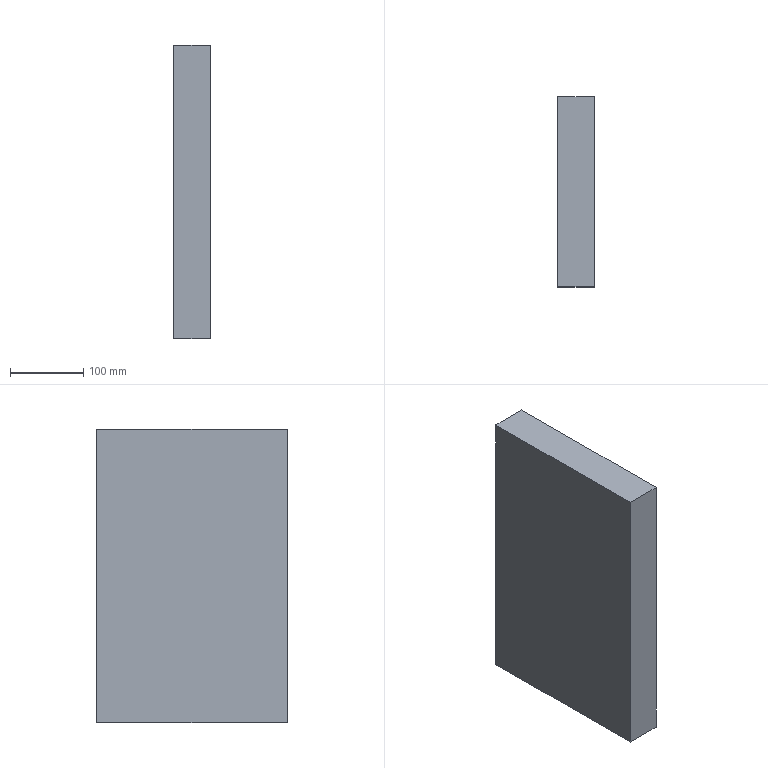Part | STEP file | 1 solid | 6 faces | box 50 x 259.164 x 400 mm | volume 5183281 mm3 | plane 6
STEP:
#1=CARTESIAN_POINT('',(0.,0.,0.));
#2=DIRECTION('',(0.,0.,1.));
#3=DIRECTION('',(1.,0.,0.));
#4=AXIS2_PLACEMENT_3D('',#1,#2,#3);
#5=CARTESIAN_POINT('',(-600.,-240.836,-56.359));
#6=VERTEX_POINT('',#5);
#7=CARTESIAN_POINT('',(-600.,-500.,-56.359));
#8=VERTEX_POINT('',#7);
#9=CARTESIAN_POINT('',(-600.,-240.836,-56.359));
#10=DIRECTION('',(0.,-1.,0.));
#11=VECTOR('',#10,1.);
#12=LINE('',#9,#11);
#13=CARTESIAN_POINT('',(-550.,-240.836,-56.359));
#14=DIRECTION('',(0.,0.,-1.));
#15=DIRECTION('',(-1.,0.,0.));
#16=AXIS2_PLACEMENT_3D('',#13,#14,#15);
#17=PLANE('',#16);
#18=CARTESIAN_POINT('',(50.,0.));
#19=DIRECTION('',(0.,-1.));
#20=VECTOR('',#19,1.);
#21=LINE('',#18,#20);
#22=(GEOMETRIC_REPRESENTATION_CONTEXT(2)PARAMETRIC_REPRESENTATION_CONTEXT()REPRESENTATION_CONTEXT('',''));
#23=DEFINITIONAL_REPRESENTATION('',(#21),#22);
#24=PCURVE('',#17,#23);
#25=CARTESIAN_POINT('',(-600.,0.,143.641));
#26=DIRECTION('',(-1.,0.,0.));
#27=DIRECTION('',(0.,0.,1.));
#28=AXIS2_PLACEMENT_3D('',#25,#26,#27);
#29=PLANE('',#28);
#30=CARTESIAN_POINT('',(-200.,-240.836));
#31=DIRECTION('',(0.,-1.));
#32=VECTOR('',#31,1.);
#33=LINE('',#30,#32);
#34=(GEOMETRIC_REPRESENTATION_CONTEXT(2)PARAMETRIC_REPRESENTATION_CONTEXT()REPRESENTATION_CONTEXT('',''));
#35=DEFINITIONAL_REPRESENTATION('',(#33),#34);
#36=PCURVE('',#29,#35);
#37=SURFACE_CURVE('',#12,(#24,#36),.PCURVE_S1.);
#38=EDGE_CURVE('',#6,#8,#37,.T.);
#39=ORIENTED_EDGE('',*,*,#38,.F.);
#40=CARTESIAN_POINT('',(-550.,-240.836,-56.359));
#41=VERTEX_POINT('',#40);
#42=CARTESIAN_POINT('',(-550.,-240.836,-56.359));
#43=DIRECTION('',(-1.,0.,0.));
#44=VECTOR('',#43,1.);
#45=LINE('',#42,#44);
#46=CARTESIAN_POINT('',(0.,0.));
#47=DIRECTION('',(1.,0.));
#48=VECTOR('',#47,1.);
#49=LINE('',#46,#48);
#50=(GEOMETRIC_REPRESENTATION_CONTEXT(2)PARAMETRIC_REPRESENTATION_CONTEXT()REPRESENTATION_CONTEXT('',''));
#51=DEFINITIONAL_REPRESENTATION('',(#49),#50);
#52=PCURVE('',#17,#51);
#53=CARTESIAN_POINT('',(-550.,-240.836,-56.359));
#54=DIRECTION('',(0.,1.,0.));
#55=DIRECTION('',(0.,0.,1.));
#56=AXIS2_PLACEMENT_3D('',#53,#54,#55);
#57=PLANE('',#56);
#58=CARTESIAN_POINT('',(0.,0.));
#59=DIRECTION('',(0.,-1.));
#60=VECTOR('',#59,1.);
#61=LINE('',#58,#60);
#62=(GEOMETRIC_REPRESENTATION_CONTEXT(2)PARAMETRIC_REPRESENTATION_CONTEXT()REPRESENTATION_CONTEXT('',''));
#63=DEFINITIONAL_REPRESENTATION('',(#61),#62);
#64=PCURVE('',#57,#63);
#65=SURFACE_CURVE('',#45,(#52,#64),.PCURVE_S1.);
#66=EDGE_CURVE('',#41,#6,#65,.T.);
#67=ORIENTED_EDGE('',*,*,#66,.F.);
#68=CARTESIAN_POINT('',(-550.,-500.,-56.359));
#69=VERTEX_POINT('',#68);
#70=CARTESIAN_POINT('',(-550.,-240.836,-56.359));
#71=DIRECTION('',(0.,-1.,0.));
#72=VECTOR('',#71,1.);
#73=LINE('',#70,#72);
#74=CARTESIAN_POINT('',(0.,0.));
#75=DIRECTION('',(0.,-1.));
#76=VECTOR('',#75,1.);
#77=LINE('',#74,#76);
#78=(GEOMETRIC_REPRESENTATION_CONTEXT(2)PARAMETRIC_REPRESENTATION_CONTEXT()REPRESENTATION_CONTEXT('',''));
#79=DEFINITIONAL_REPRESENTATION('',(#77),#78);
#80=PCURVE('',#17,#79);
#81=CARTESIAN_POINT('',(-550.,0.,143.641));
#82=DIRECTION('',(-1.,0.,0.));
#83=DIRECTION('',(0.,0.,1.));
#84=AXIS2_PLACEMENT_3D('',#81,#82,#83);
#85=PLANE('',#84);
#86=CARTESIAN_POINT('',(-200.,-240.836));
#87=DIRECTION('',(0.,-1.));
#88=VECTOR('',#87,1.);
#89=LINE('',#86,#88);
#90=(GEOMETRIC_REPRESENTATION_CONTEXT(2)PARAMETRIC_REPRESENTATION_CONTEXT()REPRESENTATION_CONTEXT('',''));
#91=DEFINITIONAL_REPRESENTATION('',(#89),#90);
#92=PCURVE('',#85,#91);
#93=SURFACE_CURVE('',#73,(#80,#92),.PCURVE_S1.);
#94=EDGE_CURVE('',#41,#69,#93,.T.);
#95=ORIENTED_EDGE('',*,*,#94,.T.);
#96=CARTESIAN_POINT('',(-550.,-500.,-56.359));
#97=DIRECTION('',(-1.,0.,0.));
#98=VECTOR('',#97,1.);
#99=LINE('',#96,#98);
#100=CARTESIAN_POINT('',(0.,-259.164));
#101=DIRECTION('',(1.,0.));
#102=VECTOR('',#101,1.);
#103=LINE('',#100,#102);
#104=(GEOMETRIC_REPRESENTATION_CONTEXT(2)PARAMETRIC_REPRESENTATION_CONTEXT()REPRESENTATION_CONTEXT('',''));
#105=DEFINITIONAL_REPRESENTATION('',(#103),#104);
#106=PCURVE('',#17,#105);
#107=CARTESIAN_POINT('',(-550.,-500.,-56.359));
#108=DIRECTION('',(0.,-1.,0.));
#109=DIRECTION('',(0.,0.,-1.));
#110=AXIS2_PLACEMENT_3D('',#107,#108,#109);
#111=PLANE('',#110);
#112=CARTESIAN_POINT('',(0.,0.));
#113=DIRECTION('',(0.,-1.));
#114=VECTOR('',#113,1.);
#115=LINE('',#112,#114);
#116=(GEOMETRIC_REPRESENTATION_CONTEXT(2)PARAMETRIC_REPRESENTATION_CONTEXT()REPRESENTATION_CONTEXT('',''));
#117=DEFINITIONAL_REPRESENTATION('',(#115),#116);
#118=PCURVE('',#111,#117);
#119=SURFACE_CURVE('',#99,(#106,#118),.PCURVE_S1.);
#120=EDGE_CURVE('',#69,#8,#119,.T.);
#121=ORIENTED_EDGE('',*,*,#120,.T.);
#122=EDGE_LOOP('',(#39,#67,#95,#121));
#123=FACE_BOUND('',#122,.T.);
#124=ADVANCED_FACE('',(#123),#17,.T.);
#125=CARTESIAN_POINT('',(-600.,-240.836,343.641));
#126=VERTEX_POINT('',#125);
#127=CARTESIAN_POINT('',(-600.,-240.836,-56.359));
#128=DIRECTION('',(0.,0.,-1.));
#129=VECTOR('',#128,1.);
#130=LINE('',#127,#129);
#131=CARTESIAN_POINT('',(0.,-50.));
#132=DIRECTION('',(-1.,0.));
#133=VECTOR('',#132,1.);
#134=LINE('',#131,#133);
#135=(GEOMETRIC_REPRESENTATION_CONTEXT(2)PARAMETRIC_REPRESENTATION_CONTEXT()REPRESENTATION_CONTEXT('',''));
#136=DEFINITIONAL_REPRESENTATION('',(#134),#135);
#137=PCURVE('',#57,#136);
#138=CARTESIAN_POINT('',(-200.,-240.836));
#139=DIRECTION('',(-1.,0.));
#140=VECTOR('',#139,1.);
#141=LINE('',#138,#140);
#142=(GEOMETRIC_REPRESENTATION_CONTEXT(2)PARAMETRIC_REPRESENTATION_CONTEXT()REPRESENTATION_CONTEXT('',''));
#143=DEFINITIONAL_REPRESENTATION('',(#141),#142);
#144=PCURVE('',#29,#143);
#145=SURFACE_CURVE('',#130,(#137,#144),.PCURVE_S1.);
#146=EDGE_CURVE('',#126,#6,#145,.T.);
#147=ORIENTED_EDGE('',*,*,#146,.F.);
#148=CARTESIAN_POINT('',(-550.,-240.836,343.641));
#149=VERTEX_POINT('',#148);
#150=CARTESIAN_POINT('',(-550.,-240.836,343.641));
#151=DIRECTION('',(-1.,0.,0.));
#152=VECTOR('',#151,1.);
#153=LINE('',#150,#152);
#154=CARTESIAN_POINT('',(400.,0.));
#155=DIRECTION('',(0.,-1.));
#156=VECTOR('',#155,1.);
#157=LINE('',#154,#156);
#158=(GEOMETRIC_REPRESENTATION_CONTEXT(2)PARAMETRIC_REPRESENTATION_CONTEXT()REPRESENTATION_CONTEXT('',''));
#159=DEFINITIONAL_REPRESENTATION('',(#157),#158);
#160=PCURVE('',#57,#159);
#161=CARTESIAN_POINT('',(-550.,-240.836,343.641));
#162=DIRECTION('',(0.,0.,1.));
#163=DIRECTION('',(1.,0.,0.));
#164=AXIS2_PLACEMENT_3D('',#161,#162,#163);
#165=PLANE('',#164);
#166=CARTESIAN_POINT('',(0.,0.));
#167=DIRECTION('',(-1.,0.));
#168=VECTOR('',#167,1.);
#169=LINE('',#166,#168);
#170=(GEOMETRIC_REPRESENTATION_CONTEXT(2)PARAMETRIC_REPRESENTATION_CONTEXT()REPRESENTATION_CONTEXT('',''));
#171=DEFINITIONAL_REPRESENTATION('',(#169),#170);
#172=PCURVE('',#165,#171);
#173=SURFACE_CURVE('',#153,(#160,#172),.PCURVE_S1.);
#174=EDGE_CURVE('',#149,#126,#173,.T.);
#175=ORIENTED_EDGE('',*,*,#174,.F.);
#176=CARTESIAN_POINT('',(-550.,-240.836,-56.359));
#177=DIRECTION('',(0.,0.,-1.));
#178=VECTOR('',#177,1.);
#179=LINE('',#176,#178);
#180=CARTESIAN_POINT('',(0.,0.));
#181=DIRECTION('',(-1.,0.));
#182=VECTOR('',#181,1.);
#183=LINE('',#180,#182);
#184=(GEOMETRIC_REPRESENTATION_CONTEXT(2)PARAMETRIC_REPRESENTATION_CONTEXT()REPRESENTATION_CONTEXT('',''));
#185=DEFINITIONAL_REPRESENTATION('',(#183),#184);
#186=PCURVE('',#57,#185);
#187=CARTESIAN_POINT('',(-200.,-240.836));
#188=DIRECTION('',(-1.,0.));
#189=VECTOR('',#188,1.);
#190=LINE('',#187,#189);
#191=(GEOMETRIC_REPRESENTATION_CONTEXT(2)PARAMETRIC_REPRESENTATION_CONTEXT()REPRESENTATION_CONTEXT('',''));
#192=DEFINITIONAL_REPRESENTATION('',(#190),#191);
#193=PCURVE('',#85,#192);
#194=SURFACE_CURVE('',#179,(#186,#193),.PCURVE_S1.);
#195=EDGE_CURVE('',#149,#41,#194,.T.);
#196=ORIENTED_EDGE('',*,*,#195,.T.);
#197=ORIENTED_EDGE('',*,*,#66,.T.);
#198=EDGE_LOOP('',(#147,#175,#196,#197));
#199=FACE_BOUND('',#198,.T.);
#200=ADVANCED_FACE('',(#199),#57,.T.);
#201=CARTESIAN_POINT('',(-600.,-500.,343.641));
#202=VERTEX_POINT('',#201);
#203=CARTESIAN_POINT('',(-600.,-240.836,343.641));
#204=DIRECTION('',(0.,1.,0.));
#205=VECTOR('',#204,1.);
#206=LINE('',#203,#205);
#207=CARTESIAN_POINT('',(-50.,0.));
#208=DIRECTION('',(0.,1.));
#209=VECTOR('',#208,1.);
#210=LINE('',#207,#209);
#211=(GEOMETRIC_REPRESENTATION_CONTEXT(2)PARAMETRIC_REPRESENTATION_CONTEXT()REPRESENTATION_CONTEXT('',''));
#212=DEFINITIONAL_REPRESENTATION('',(#210),#211);
#213=PCURVE('',#165,#212);
#214=CARTESIAN_POINT('',(200.,-240.836));
#215=DIRECTION('',(0.,1.));
#216=VECTOR('',#215,1.);
#217=LINE('',#214,#216);
#218=(GEOMETRIC_REPRESENTATION_CONTEXT(2)PARAMETRIC_REPRESENTATION_CONTEXT()REPRESENTATION_CONTEXT('',''));
#219=DEFINITIONAL_REPRESENTATION('',(#217),#218);
#220=PCURVE('',#29,#219);
#221=SURFACE_CURVE('',#206,(#213,#220),.PCURVE_S1.);
#222=EDGE_CURVE('',#202,#126,#221,.T.);
#223=ORIENTED_EDGE('',*,*,#222,.F.);
#224=CARTESIAN_POINT('',(-550.,-500.,343.641));
#225=VERTEX_POINT('',#224);
#226=CARTESIAN_POINT('',(-550.,-500.,343.641));
#227=DIRECTION('',(-1.,0.,0.));
#228=VECTOR('',#227,1.);
#229=LINE('',#226,#228);
#230=CARTESIAN_POINT('',(0.,-259.164));
#231=DIRECTION('',(-1.,0.));
#232=VECTOR('',#231,1.);
#233=LINE('',#230,#232);
#234=(GEOMETRIC_REPRESENTATION_CONTEXT(2)PARAMETRIC_REPRESENTATION_CONTEXT()REPRESENTATION_CONTEXT('',''));
#235=DEFINITIONAL_REPRESENTATION('',(#233),#234);
#236=PCURVE('',#165,#235);
#237=CARTESIAN_POINT('',(-400.,0.));
#238=DIRECTION('',(0.,-1.));
#239=VECTOR('',#238,1.);
#240=LINE('',#237,#239);
#241=(GEOMETRIC_REPRESENTATION_CONTEXT(2)PARAMETRIC_REPRESENTATION_CONTEXT()REPRESENTATION_CONTEXT('',''));
#242=DEFINITIONAL_REPRESENTATION('',(#240),#241);
#243=PCURVE('',#111,#242);
#244=SURFACE_CURVE('',#229,(#236,#243),.PCURVE_S1.);
#245=EDGE_CURVE('',#225,#202,#244,.T.);
#246=ORIENTED_EDGE('',*,*,#245,.F.);
#247=CARTESIAN_POINT('',(-550.,-240.836,343.641));
#248=DIRECTION('',(0.,1.,0.));
#249=VECTOR('',#248,1.);
#250=LINE('',#247,#249);
#251=CARTESIAN_POINT('',(0.,0.));
#252=DIRECTION('',(0.,1.));
#253=VECTOR('',#252,1.);
#254=LINE('',#251,#253);
#255=(GEOMETRIC_REPRESENTATION_CONTEXT(2)PARAMETRIC_REPRESENTATION_CONTEXT()REPRESENTATION_CONTEXT('',''));
#256=DEFINITIONAL_REPRESENTATION('',(#254),#255);
#257=PCURVE('',#165,#256);
#258=CARTESIAN_POINT('',(200.,-240.836));
#259=DIRECTION('',(0.,1.));
#260=VECTOR('',#259,1.);
#261=LINE('',#258,#260);
#262=(GEOMETRIC_REPRESENTATION_CONTEXT(2)PARAMETRIC_REPRESENTATION_CONTEXT()REPRESENTATION_CONTEXT('',''));
#263=DEFINITIONAL_REPRESENTATION('',(#261),#262);
#264=PCURVE('',#85,#263);
#265=SURFACE_CURVE('',#250,(#257,#264),.PCURVE_S1.);
#266=EDGE_CURVE('',#225,#149,#265,.T.);
#267=ORIENTED_EDGE('',*,*,#266,.T.);
#268=ORIENTED_EDGE('',*,*,#174,.T.);
#269=EDGE_LOOP('',(#223,#246,#267,#268));
#270=FACE_BOUND('',#269,.T.);
#271=ADVANCED_FACE('',(#270),#165,.T.);
#272=CARTESIAN_POINT('',(-600.,-500.,-56.359));
#273=DIRECTION('',(0.,0.,1.));
#274=VECTOR('',#273,1.);
#275=LINE('',#272,#274);
#276=CARTESIAN_POINT('',(0.,-50.));
#277=DIRECTION('',(-1.,0.));
#278=VECTOR('',#277,1.);
#279=LINE('',#276,#278);
#280=(GEOMETRIC_REPRESENTATION_CONTEXT(2)PARAMETRIC_REPRESENTATION_CONTEXT()REPRESENTATION_CONTEXT('',''));
#281=DEFINITIONAL_REPRESENTATION('',(#279),#280);
#282=PCURVE('',#111,#281);
#283=CARTESIAN_POINT('',(-200.,-500.));
#284=DIRECTION('',(1.,0.));
#285=VECTOR('',#284,1.);
#286=LINE('',#283,#285);
#287=(GEOMETRIC_REPRESENTATION_CONTEXT(2)PARAMETRIC_REPRESENTATION_CONTEXT()REPRESENTATION_CONTEXT('',''));
#288=DEFINITIONAL_REPRESENTATION('',(#286),#287);
#289=PCURVE('',#29,#288);
#290=SURFACE_CURVE('',#275,(#282,#289),.PCURVE_S1.);
#291=EDGE_CURVE('',#8,#202,#290,.T.);
#292=ORIENTED_EDGE('',*,*,#291,.F.);
#293=ORIENTED_EDGE('',*,*,#120,.F.);
#294=CARTESIAN_POINT('',(-550.,-500.,-56.359));
#295=DIRECTION('',(0.,0.,1.));
#296=VECTOR('',#295,1.);
#297=LINE('',#294,#296);
#298=CARTESIAN_POINT('',(0.,0.));
#299=DIRECTION('',(-1.,0.));
#300=VECTOR('',#299,1.);
#301=LINE('',#298,#300);
#302=(GEOMETRIC_REPRESENTATION_CONTEXT(2)PARAMETRIC_REPRESENTATION_CONTEXT()REPRESENTATION_CONTEXT('',''));
#303=DEFINITIONAL_REPRESENTATION('',(#301),#302);
#304=PCURVE('',#111,#303);
#305=CARTESIAN_POINT('',(-200.,-500.));
#306=DIRECTION('',(1.,0.));
#307=VECTOR('',#306,1.);
#308=LINE('',#305,#307);
#309=(GEOMETRIC_REPRESENTATION_CONTEXT(2)PARAMETRIC_REPRESENTATION_CONTEXT()REPRESENTATION_CONTEXT('',''));
#310=DEFINITIONAL_REPRESENTATION('',(#308),#309);
#311=PCURVE('',#85,#310);
#312=SURFACE_CURVE('',#297,(#304,#311),.PCURVE_S1.);
#313=EDGE_CURVE('',#69,#225,#312,.T.);
#314=ORIENTED_EDGE('',*,*,#313,.T.);
#315=ORIENTED_EDGE('',*,*,#245,.T.);
#316=EDGE_LOOP('',(#292,#293,#314,#315));
#317=FACE_BOUND('',#316,.T.);
#318=ADVANCED_FACE('',(#317),#111,.T.);
#319=ORIENTED_EDGE('',*,*,#94,.F.);
#320=ORIENTED_EDGE('',*,*,#195,.F.);
#321=ORIENTED_EDGE('',*,*,#266,.F.);
#322=ORIENTED_EDGE('',*,*,#313,.F.);
#323=EDGE_LOOP('',(#319,#320,#321,#322));
#324=FACE_BOUND('',#323,.T.);
#325=ADVANCED_FACE('',(#324),#85,.F.);
#326=ORIENTED_EDGE('',*,*,#38,.T.);
#327=ORIENTED_EDGE('',*,*,#291,.T.);
#328=ORIENTED_EDGE('',*,*,#222,.T.);
#329=ORIENTED_EDGE('',*,*,#146,.T.);
#330=EDGE_LOOP('',(#326,#327,#328,#329));
#331=FACE_BOUND('',#330,.T.);
#332=ADVANCED_FACE('',(#331),#29,.T.);
#333=CLOSED_SHELL('',(#124,#200,#271,#318,#325,#332));
#334=MANIFOLD_SOLID_BREP('',#333);
#335=(LENGTH_UNIT()NAMED_UNIT(*)SI_UNIT(.MILLI.,.METRE.));
#336=UNCERTAINTY_MEASURE_WITH_UNIT(LENGTH_MEASURE(0.0000001),#335,'','');
#337=(NAMED_UNIT(*)PLANE_ANGLE_UNIT()SI_UNIT($,.RADIAN.));
#338=(NAMED_UNIT(*)SI_UNIT($,.STERADIAN.)SOLID_ANGLE_UNIT());
#339=(GEOMETRIC_REPRESENTATION_CONTEXT(3)GLOBAL_UNCERTAINTY_ASSIGNED_CONTEXT((#336))GLOBAL_UNIT_ASSIGNED_CONTEXT((#335,#337,#338))REPRESENTATION_CONTEXT('',''));
#340=ADVANCED_BREP_SHAPE_REPRESENTATION('',(#4,#334),#339);